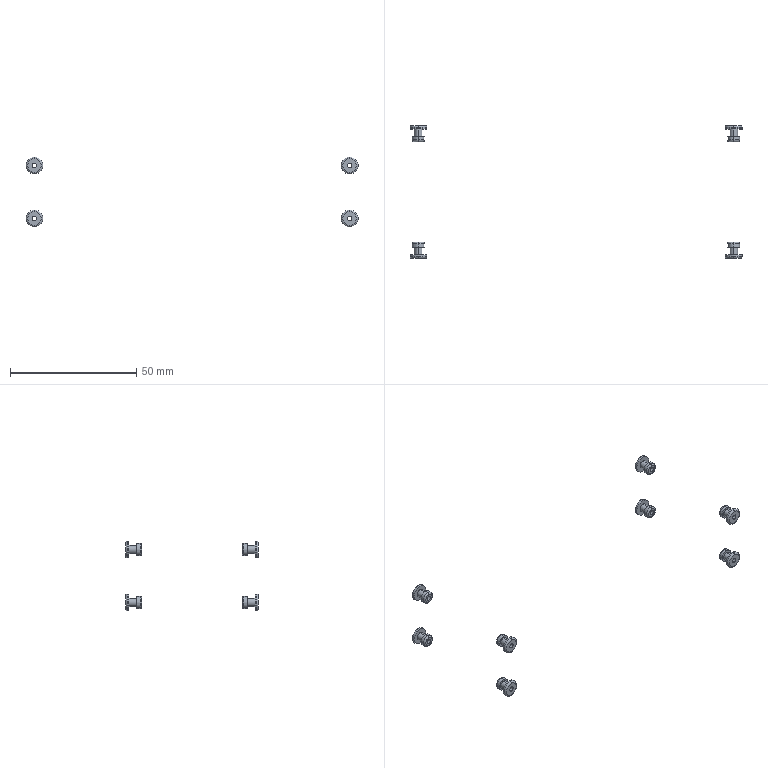Part | STEP file | Rebite cego ISO 15973 - d3.2-6.5. | 8 solids | 128 faces | box 131.7 x 52.6 x 27.7 mm | volume 686.978 mm3 | cylinder 64 | torus 32 | plane 32 | commonest cylinder face diameters 1.85 x16 3.2 x16 4.8 x16 6.7 x16